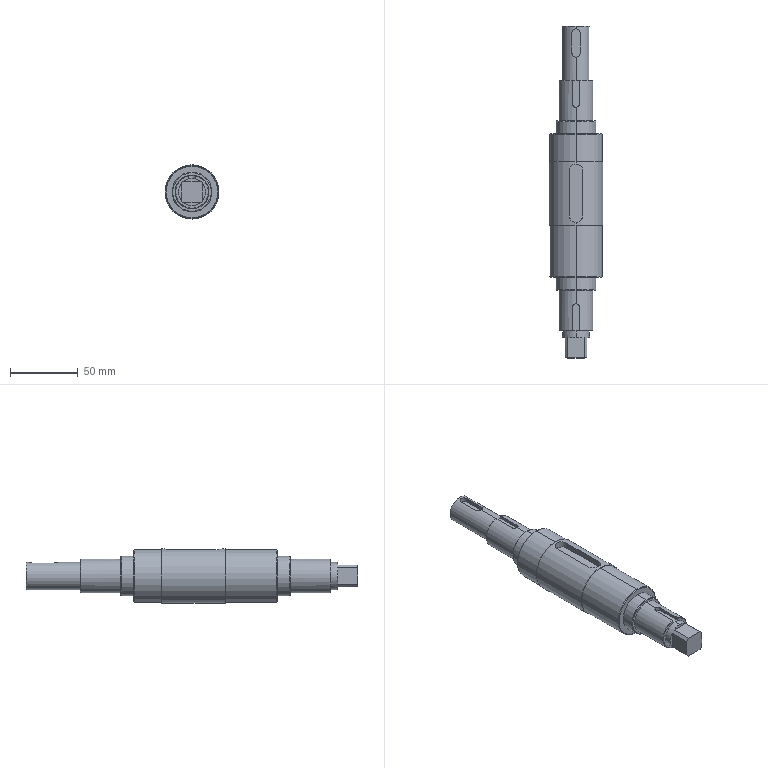Part | SolidWorks | features Boss 7, Chamfer 3, ICE 3, Cut 2, Extrusion 1 | 1 solid | 68 faces | box 40 x 245 x 40 mm | volume 186940 mm3 | plane 30 | cylinder 25 | cone 13 | commonest cylinder face diameters 20 x4 25 x4 29.5 x4 39 x4 5 x2 6 x2